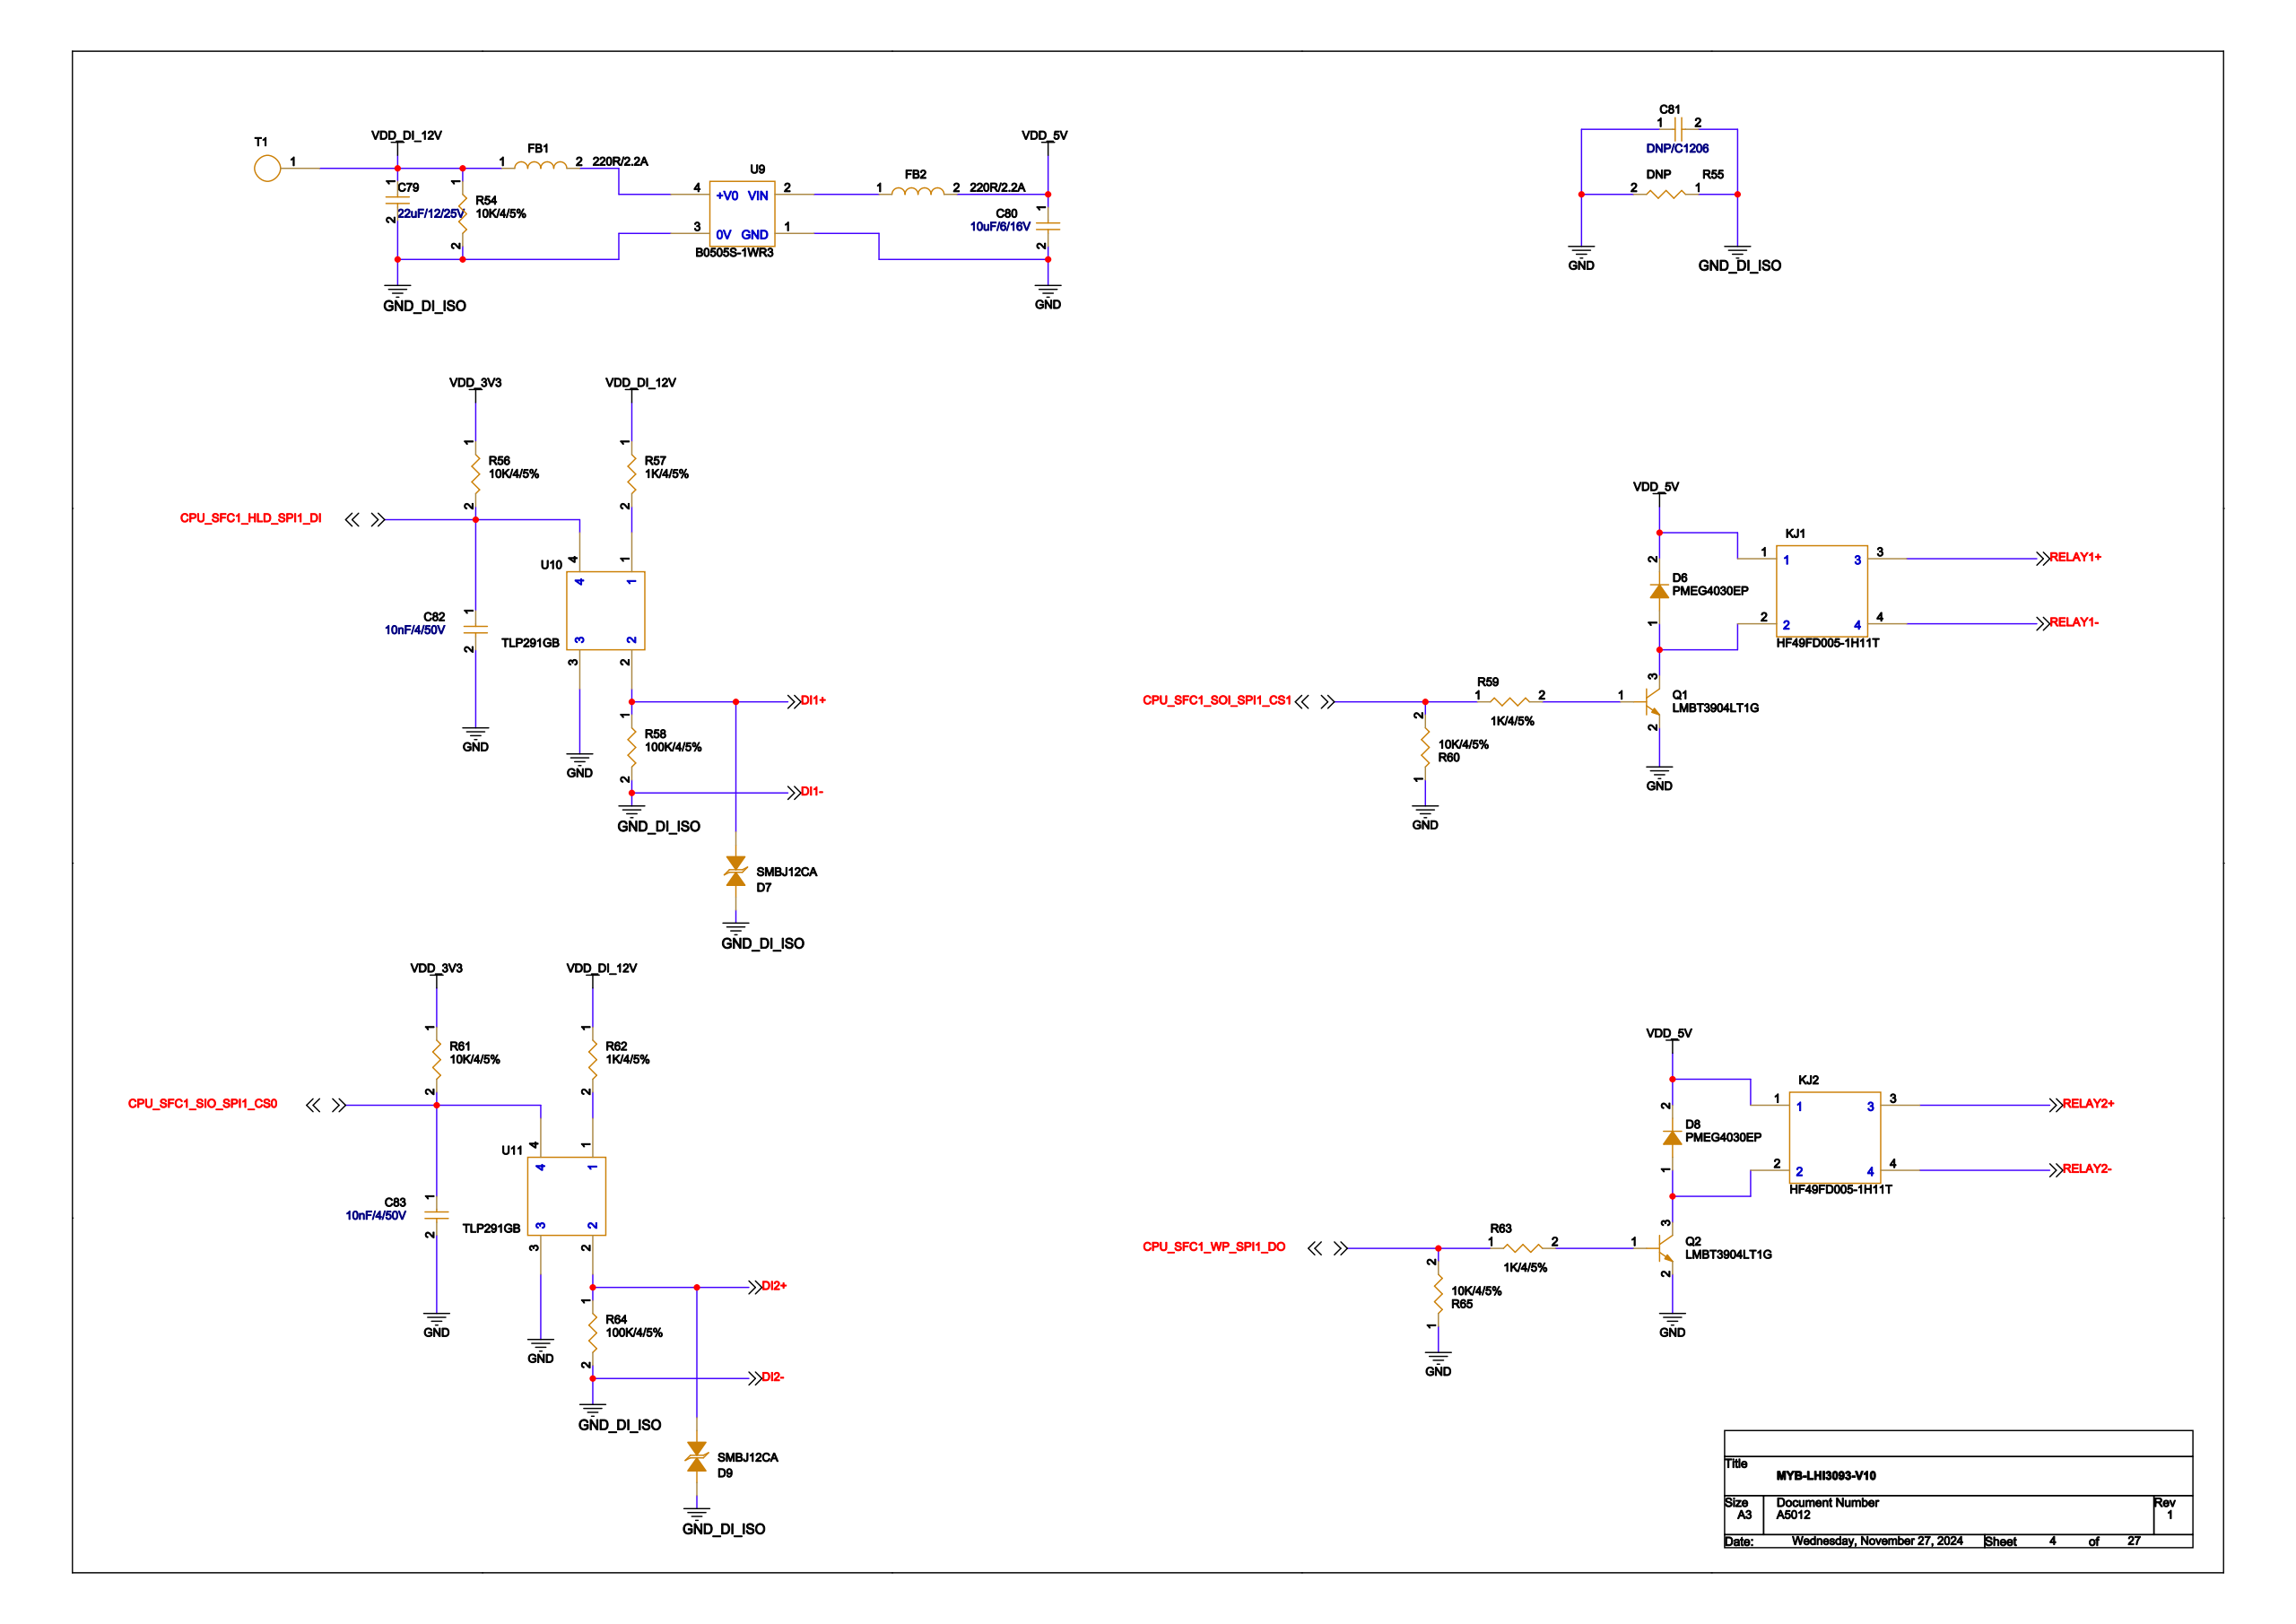Circuit board | Cadence Allegro | 1159 parts | 708 nets | one sheet of the schematic
Parts on this sheet (reference | value | footprint):
C79 | 22uF/12/25V | C1206
C80 | 10uF/6/16V | C0603
C81 | DNP/C1206 | C1206
C82 | 10nF/4/50V | C0402
C83 | 10nF/4/50V | C0402
D6 | PMEG4030EP | DO-214AA
D7 | SMBJ12CA | DO-214AA
D8 | PMEG4030EP | DO-214AA
D9 | SMBJ12CA | DO-214AA
FB1 | 220R/2.2A | FB0603
FB2 | 220R/2.2A | FB0603
KJ1 | HF49FD005-1H11T | RELAY-HF49FD005-1H11T
KJ2 | HF49FD005-1H11T | RELAY-HF49FD005-1H11T
Q1 | LMBT3904LT1G | SOT-23
Q2 | LMBT3904LT1G | SOT-23
R54 | 10K/4/5% | R0402
R55 | DNP | R1206
R56 | 10K/4/5% | R0402
R57 | 1K/4/5% | R0402
R58 | 100K/4/5% | R0402
R59 | 1K/4/5% | R0402
R60 | 10K/4/5% | R0402
R61 | 10K/4/5% | R0402
R62 | 1K/4/5% | R0402
R63 | 1K/4/5% | R0402
R64 | 100K/4/5% | R0402
R65 | 10K/4/5% | R0402
T1 | SMD | TP_SMT
U9 | B0505S-1WR3 | MODULE-B0512S
U10 | TLP291GB | TLP281
U11 | TLP291GB | TLP281
Nets of these parts (net: part-pin ...):
GND: C80-2 C81-1 C82-2 C83-2 Q1-2 Q2-2 R55-2 R60-1 R65-1 U9-1 U10-3 U11-3
VDD_5V: C80-1 D6-2 D8-2 FB2-2 KJ1-1 KJ2-1
VDD_DI_12V: C79-1 FB1-1 R54-1 R57-1 R62-1 T1-1
DI1-: C79-2 C81-2 D7-1 D9-1 R54-2 R55-1 R58-2 R64-2 U9-3
VDD_3V3: R56-1 R61-1
CPU_SFC1_HLD_SPI1_DI: C82-1 R56-2 U10-4
CPU_SFC1_SIO_SPI1_CS0: C83-1 R61-2 U11-4
DI1+: D7-2 R58-1 U10-2
DI2+: D9-2 R64-1 U11-2
N14933893: D6-1 KJ1-2 Q1-3
N14934578: D8-1 KJ2-2 Q2-3
N14933263: FB1-2 U9-4
N14933596: FB2-1 U9-2
RELAY1+: KJ1-3
RELAY1-: KJ1-4
RELAY2+: KJ2-3
RELAY2-: KJ2-4
N14934143: Q1-1 R59-2
N14934680: Q2-1 R63-2
CPU_SFC1_SOI_SPI1_CS1: R59-1 R60-2
CPU_SFC1_WP_SPI1_DO: R63-1 R65-2
N14935253: R57-2 U10-1
N14936339: R62-2 U11-1